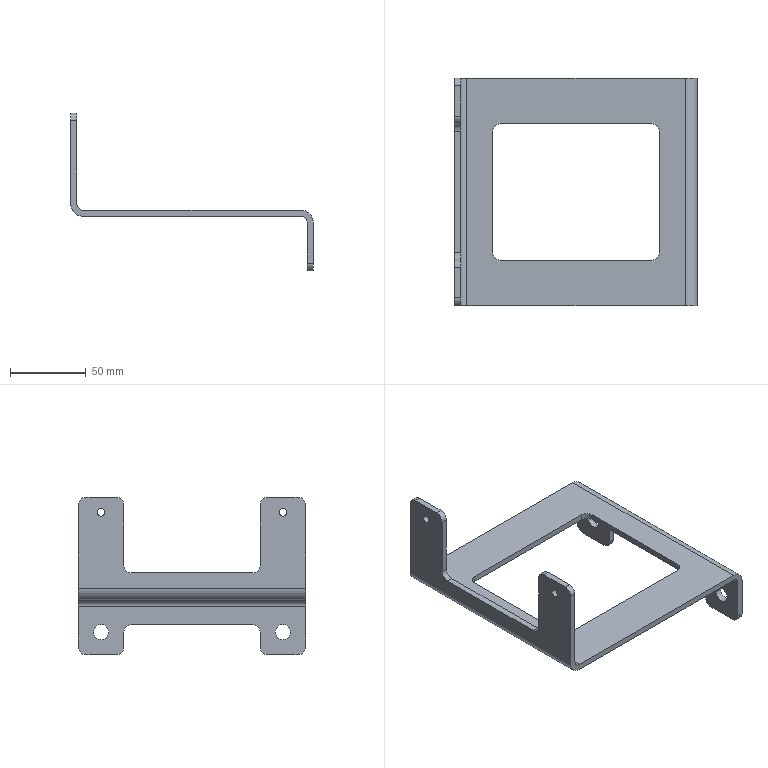Part | STEP file | J452-EBZ05-24-08 | 1 solid | 50 faces | box 160 x 150 x 104 mm | volume 87324 mm3 | cylinder 28 | plane 22 | commonest cylinder face diameters 10 x20 5 x4 8 x2 16 x2